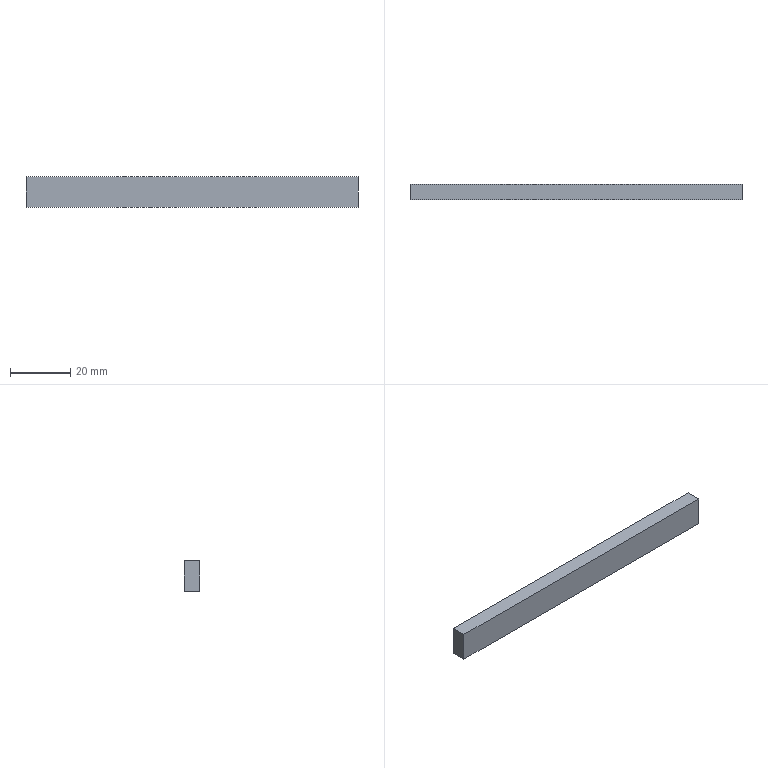Part | SolidWorks | features Extrusion 1, ICE 1 | 1 solid | 12 faces | box 110 x 5 x 10 mm | volume 5325 mm3 | plane 8 | cylinder 4 | commonest cylinder face diameters 6 x4
STEP:
#1=CARTESIAN_POINT('',(-49.,1.9,-3.));
#2=VERTEX_POINT('',#1);
#3=CARTESIAN_POINT('',(-49.,1.9,3.));
#4=VERTEX_POINT('',#3);
#5=CARTESIAN_POINT('',(-49.,1.9,0.));
#6=DIRECTION('',(0.,1.,0.));
#7=DIRECTION('',(0.,0.,1.));
#8=AXIS2_PLACEMENT_3D('',#5,#6,#7);
#9=CIRCLE('',#8,3.);
#10=EDGE_CURVE('',#2,#4,#9,.T.);
#11=ORIENTED_EDGE('',*,*,#10,.F.);
#12=CARTESIAN_POINT('',(-49.,5.,-3.));
#13=VERTEX_POINT('',#12);
#14=CARTESIAN_POINT('',(-49.,1.9,-3.));
#15=DIRECTION('',(0.,1.,0.));
#16=VECTOR('',#15,1000.);
#17=LINE('',#14,#16);
#18=EDGE_CURVE('',#2,#13,#17,.T.);
#19=ORIENTED_EDGE('',*,*,#18,.T.);
#20=CARTESIAN_POINT('',(-49.,5.,3.));
#21=VERTEX_POINT('',#20);
#22=CARTESIAN_POINT('',(-49.,5.,0.));
#23=DIRECTION('',(0.,1.,0.));
#24=DIRECTION('',(0.,0.,1.));
#25=AXIS2_PLACEMENT_3D('',#22,#23,#24);
#26=CIRCLE('',#25,3.);
#27=EDGE_CURVE('',#13,#21,#26,.T.);
#28=ORIENTED_EDGE('',*,*,#27,.T.);
#29=CARTESIAN_POINT('',(-49.,1.9,3.));
#30=DIRECTION('',(0.,1.,0.));
#31=VECTOR('',#30,1000.);
#32=LINE('',#29,#31);
#33=EDGE_CURVE('',#4,#21,#32,.T.);
#34=ORIENTED_EDGE('',*,*,#33,.F.);
#35=EDGE_LOOP('',(#11,#19,#28,#34));
#36=FACE_OUTER_BOUND('',#35,.T.);
#37=CARTESIAN_POINT('',(-49.,1.9,0.));
#38=DIRECTION('',(0.,1.,0.));
#39=DIRECTION('',(0.,0.,1.));
#40=AXIS2_PLACEMENT_3D('',#37,#38,#39);
#41=CYLINDRICAL_SURFACE('',#40,3.);
#42=ADVANCED_FACE('',(#36),#41,.F.);
#43=CARTESIAN_POINT('',(49.,1.9,-3.));
#44=VERTEX_POINT('',#43);
#45=CARTESIAN_POINT('',(49.,1.9,3.));
#46=VERTEX_POINT('',#45);
#47=CARTESIAN_POINT('',(49.,1.9,0.));
#48=DIRECTION('',(0.,1.,0.));
#49=DIRECTION('',(0.,0.,1.));
#50=AXIS2_PLACEMENT_3D('',#47,#48,#49);
#51=CIRCLE('',#50,3.);
#52=EDGE_CURVE('',#44,#46,#51,.T.);
#53=ORIENTED_EDGE('',*,*,#52,.F.);
#54=CARTESIAN_POINT('',(49.,5.,-3.));
#55=VERTEX_POINT('',#54);
#56=CARTESIAN_POINT('',(49.,1.9,-3.));
#57=DIRECTION('',(0.,1.,0.));
#58=VECTOR('',#57,1000.);
#59=LINE('',#56,#58);
#60=EDGE_CURVE('',#44,#55,#59,.T.);
#61=ORIENTED_EDGE('',*,*,#60,.T.);
#62=CARTESIAN_POINT('',(49.,5.,3.));
#63=VERTEX_POINT('',#62);
#64=CARTESIAN_POINT('',(49.,5.,0.));
#65=DIRECTION('',(0.,1.,0.));
#66=DIRECTION('',(0.,0.,1.));
#67=AXIS2_PLACEMENT_3D('',#64,#65,#66);
#68=CIRCLE('',#67,3.);
#69=EDGE_CURVE('',#55,#63,#68,.T.);
#70=ORIENTED_EDGE('',*,*,#69,.T.);
#71=CARTESIAN_POINT('',(49.,1.9,3.));
#72=DIRECTION('',(0.,1.,0.));
#73=VECTOR('',#72,1000.);
#74=LINE('',#71,#73);
#75=EDGE_CURVE('',#46,#63,#74,.T.);
#76=ORIENTED_EDGE('',*,*,#75,.F.);
#77=EDGE_LOOP('',(#53,#61,#70,#76));
#78=FACE_OUTER_BOUND('',#77,.T.);
#79=CARTESIAN_POINT('',(49.,1.9,0.));
#80=DIRECTION('',(0.,1.,0.));
#81=DIRECTION('',(0.,0.,1.));
#82=AXIS2_PLACEMENT_3D('',#79,#80,#81);
#83=CYLINDRICAL_SURFACE('',#82,3.);
#84=ADVANCED_FACE('',(#78),#83,.F.);
#85=CARTESIAN_POINT('',(55.,0.,5.));
#86=VERTEX_POINT('',#85);
#87=CARTESIAN_POINT('',(55.,0.,-5.));
#88=VERTEX_POINT('',#87);
#89=CARTESIAN_POINT('',(55.,0.,-5.));
#90=DIRECTION('',(0.,0.,-1.));
#91=VECTOR('',#90,1000.);
#92=LINE('',#89,#91);
#93=EDGE_CURVE('',#86,#88,#92,.T.);
#94=ORIENTED_EDGE('',*,*,#93,.T.);
#95=CARTESIAN_POINT('',(55.,5.,-5.));
#96=VERTEX_POINT('',#95);
#97=CARTESIAN_POINT('',(55.,5.,-5.));
#98=DIRECTION('',(0.,-1.,0.));
#99=VECTOR('',#98,1000.);
#100=LINE('',#97,#99);
#101=EDGE_CURVE('',#96,#88,#100,.T.);
#102=ORIENTED_EDGE('',*,*,#101,.F.);
#103=CARTESIAN_POINT('',(55.,5.,5.));
#104=VERTEX_POINT('',#103);
#105=CARTESIAN_POINT('',(55.,5.,-5.));
#106=DIRECTION('',(0.,0.,-1.));
#107=VECTOR('',#106,1000.);
#108=LINE('',#105,#107);
#109=EDGE_CURVE('',#104,#96,#108,.T.);
#110=ORIENTED_EDGE('',*,*,#109,.F.);
#111=CARTESIAN_POINT('',(55.,5.,5.));
#112=DIRECTION('',(0.,-1.,0.));
#113=VECTOR('',#112,1000.);
#114=LINE('',#111,#113);
#115=EDGE_CURVE('',#104,#86,#114,.T.);
#116=ORIENTED_EDGE('',*,*,#115,.T.);
#117=EDGE_LOOP('',(#94,#102,#110,#116));
#118=FACE_OUTER_BOUND('',#117,.T.);
#119=CARTESIAN_POINT('',(55.,5.,-5.));
#120=DIRECTION('',(-1.,0.,0.));
#121=DIRECTION('',(0.,0.,1.));
#122=AXIS2_PLACEMENT_3D('',#119,#120,#121);
#123=PLANE('',#122);
#124=ADVANCED_FACE('',(#118),#123,.F.);
#125=CARTESIAN_POINT('',(-55.,0.,-5.));
#126=VERTEX_POINT('',#125);
#127=CARTESIAN_POINT('',(-55.,0.,-5.));
#128=DIRECTION('',(-1.,0.,0.));
#129=VECTOR('',#128,1000.);
#130=LINE('',#127,#129);
#131=EDGE_CURVE('',#88,#126,#130,.T.);
#132=ORIENTED_EDGE('',*,*,#131,.T.);
#133=CARTESIAN_POINT('',(-55.,5.,-5.));
#134=VERTEX_POINT('',#133);
#135=CARTESIAN_POINT('',(-55.,5.,-5.));
#136=DIRECTION('',(0.,-1.,0.));
#137=VECTOR('',#136,1000.);
#138=LINE('',#135,#137);
#139=EDGE_CURVE('',#134,#126,#138,.T.);
#140=ORIENTED_EDGE('',*,*,#139,.F.);
#141=CARTESIAN_POINT('',(-55.,5.,-5.));
#142=DIRECTION('',(-1.,0.,0.));
#143=VECTOR('',#142,1000.);
#144=LINE('',#141,#143);
#145=EDGE_CURVE('',#96,#134,#144,.T.);
#146=ORIENTED_EDGE('',*,*,#145,.F.);
#147=ORIENTED_EDGE('',*,*,#101,.T.);
#148=EDGE_LOOP('',(#132,#140,#146,#147));
#149=FACE_OUTER_BOUND('',#148,.T.);
#150=CARTESIAN_POINT('',(-55.,5.,-5.));
#151=DIRECTION('',(0.,0.,1.));
#152=DIRECTION('',(1.,0.,0.));
#153=AXIS2_PLACEMENT_3D('',#150,#151,#152);
#154=PLANE('',#153);
#155=ADVANCED_FACE('',(#149),#154,.F.);
#156=CARTESIAN_POINT('',(-55.,0.,5.));
#157=VERTEX_POINT('',#156);
#158=CARTESIAN_POINT('',(-55.,0.,-5.));
#159=DIRECTION('',(0.,0.,1.));
#160=VECTOR('',#159,1000.);
#161=LINE('',#158,#160);
#162=EDGE_CURVE('',#126,#157,#161,.T.);
#163=ORIENTED_EDGE('',*,*,#162,.T.);
#164=CARTESIAN_POINT('',(-55.,5.,5.));
#165=VERTEX_POINT('',#164);
#166=CARTESIAN_POINT('',(-55.,5.,5.));
#167=DIRECTION('',(0.,-1.,0.));
#168=VECTOR('',#167,1000.);
#169=LINE('',#166,#168);
#170=EDGE_CURVE('',#165,#157,#169,.T.);
#171=ORIENTED_EDGE('',*,*,#170,.F.);
#172=CARTESIAN_POINT('',(-55.,5.,-5.));
#173=DIRECTION('',(0.,0.,1.));
#174=VECTOR('',#173,1000.);
#175=LINE('',#172,#174);
#176=EDGE_CURVE('',#134,#165,#175,.T.);
#177=ORIENTED_EDGE('',*,*,#176,.F.);
#178=ORIENTED_EDGE('',*,*,#139,.T.);
#179=EDGE_LOOP('',(#163,#171,#177,#178));
#180=FACE_OUTER_BOUND('',#179,.T.);
#181=CARTESIAN_POINT('',(-55.,5.,-5.));
#182=DIRECTION('',(1.,0.,0.));
#183=DIRECTION('',(0.,0.,-1.));
#184=AXIS2_PLACEMENT_3D('',#181,#182,#183);
#185=PLANE('',#184);
#186=ADVANCED_FACE('',(#180),#185,.F.);
#187=CARTESIAN_POINT('',(-55.,0.,5.));
#188=DIRECTION('',(1.,0.,0.));
#189=VECTOR('',#188,1000.);
#190=LINE('',#187,#189);
#191=EDGE_CURVE('',#157,#86,#190,.T.);
#192=ORIENTED_EDGE('',*,*,#191,.T.);
#193=ORIENTED_EDGE('',*,*,#115,.F.);
#194=CARTESIAN_POINT('',(-55.,5.,5.));
#195=DIRECTION('',(1.,0.,0.));
#196=VECTOR('',#195,1000.);
#197=LINE('',#194,#196);
#198=EDGE_CURVE('',#165,#104,#197,.T.);
#199=ORIENTED_EDGE('',*,*,#198,.F.);
#200=ORIENTED_EDGE('',*,*,#170,.T.);
#201=EDGE_LOOP('',(#192,#193,#199,#200));
#202=FACE_OUTER_BOUND('',#201,.T.);
#203=CARTESIAN_POINT('',(-55.,5.,5.));
#204=DIRECTION('',(0.,0.,-1.));
#205=DIRECTION('',(-1.,0.,0.));
#206=AXIS2_PLACEMENT_3D('',#203,#204,#205);
#207=PLANE('',#206);
#208=ADVANCED_FACE('',(#202),#207,.F.);
#209=CARTESIAN_POINT('',(-49.,5.,0.));
#210=DIRECTION('',(0.,1.,0.));
#211=DIRECTION('',(0.,0.,1.));
#212=AXIS2_PLACEMENT_3D('',#209,#210,#211);
#213=CIRCLE('',#212,3.);
#214=EDGE_CURVE('',#21,#13,#213,.T.);
#215=ORIENTED_EDGE('',*,*,#214,.F.);
#216=ORIENTED_EDGE('',*,*,#27,.F.);
#217=EDGE_LOOP('',(#215,#216));
#218=FACE_BOUND('',#217,.T.);
#219=CARTESIAN_POINT('',(49.,5.,0.));
#220=DIRECTION('',(0.,1.,0.));
#221=DIRECTION('',(0.,0.,1.));
#222=AXIS2_PLACEMENT_3D('',#219,#220,#221);
#223=CIRCLE('',#222,3.);
#224=EDGE_CURVE('',#63,#55,#223,.T.);
#225=ORIENTED_EDGE('',*,*,#224,.F.);
#226=ORIENTED_EDGE('',*,*,#69,.F.);
#227=EDGE_LOOP('',(#225,#226));
#228=FACE_BOUND('',#227,.T.);
#229=ORIENTED_EDGE('',*,*,#109,.T.);
#230=ORIENTED_EDGE('',*,*,#145,.T.);
#231=ORIENTED_EDGE('',*,*,#176,.T.);
#232=ORIENTED_EDGE('',*,*,#198,.T.);
#233=EDGE_LOOP('',(#229,#230,#231,#232));
#234=FACE_OUTER_BOUND('',#233,.T.);
#235=CARTESIAN_POINT('',(0.,5.,0.));
#236=DIRECTION('',(0.,1.,0.));
#237=DIRECTION('',(0.,0.,1.));
#238=AXIS2_PLACEMENT_3D('',#235,#236,#237);
#239=PLANE('',#238);
#240=ADVANCED_FACE('',(#218,#228,#234),#239,.T.);
#241=ORIENTED_EDGE('',*,*,#93,.F.);
#242=ORIENTED_EDGE('',*,*,#191,.F.);
#243=ORIENTED_EDGE('',*,*,#162,.F.);
#244=ORIENTED_EDGE('',*,*,#131,.F.);
#245=EDGE_LOOP('',(#241,#242,#243,#244));
#246=FACE_OUTER_BOUND('',#245,.T.);
#247=CARTESIAN_POINT('',(0.,0.,0.));
#248=DIRECTION('',(0.,1.,0.));
#249=DIRECTION('',(0.,0.,1.));
#250=AXIS2_PLACEMENT_3D('',#247,#248,#249);
#251=PLANE('',#250);
#252=ADVANCED_FACE('',(#246),#251,.F.);
#253=ORIENTED_EDGE('',*,*,#60,.F.);
#254=CARTESIAN_POINT('',(49.,1.9,0.));
#255=DIRECTION('',(0.,1.,0.));
#256=DIRECTION('',(0.,0.,1.));
#257=AXIS2_PLACEMENT_3D('',#254,#255,#256);
#258=CIRCLE('',#257,3.);
#259=EDGE_CURVE('',#46,#44,#258,.T.);
#260=ORIENTED_EDGE('',*,*,#259,.F.);
#261=ORIENTED_EDGE('',*,*,#75,.T.);
#262=ORIENTED_EDGE('',*,*,#224,.T.);
#263=EDGE_LOOP('',(#253,#260,#261,#262));
#264=FACE_OUTER_BOUND('',#263,.T.);
#265=CARTESIAN_POINT('',(49.,1.9,0.));
#266=DIRECTION('',(0.,1.,0.));
#267=DIRECTION('',(0.,0.,1.));
#268=AXIS2_PLACEMENT_3D('',#265,#266,#267);
#269=CYLINDRICAL_SURFACE('',#268,3.);
#270=ADVANCED_FACE('',(#264),#269,.F.);
#271=ORIENTED_EDGE('',*,*,#259,.T.);
#272=ORIENTED_EDGE('',*,*,#52,.T.);
#273=EDGE_LOOP('',(#271,#272));
#274=FACE_OUTER_BOUND('',#273,.T.);
#275=CARTESIAN_POINT('',(49.,1.9,0.));
#276=DIRECTION('',(0.,1.,0.));
#277=DIRECTION('',(0.,0.,1.));
#278=AXIS2_PLACEMENT_3D('',#275,#276,#277);
#279=PLANE('',#278);
#280=ADVANCED_FACE('',(#274),#279,.T.);
#281=ORIENTED_EDGE('',*,*,#18,.F.);
#282=CARTESIAN_POINT('',(-49.,1.9,0.));
#283=DIRECTION('',(0.,1.,0.));
#284=DIRECTION('',(0.,0.,1.));
#285=AXIS2_PLACEMENT_3D('',#282,#283,#284);
#286=CIRCLE('',#285,3.);
#287=EDGE_CURVE('',#4,#2,#286,.T.);
#288=ORIENTED_EDGE('',*,*,#287,.F.);
#289=ORIENTED_EDGE('',*,*,#33,.T.);
#290=ORIENTED_EDGE('',*,*,#214,.T.);
#291=EDGE_LOOP('',(#281,#288,#289,#290));
#292=FACE_OUTER_BOUND('',#291,.T.);
#293=CARTESIAN_POINT('',(-49.,1.9,0.));
#294=DIRECTION('',(0.,1.,0.));
#295=DIRECTION('',(0.,0.,1.));
#296=AXIS2_PLACEMENT_3D('',#293,#294,#295);
#297=CYLINDRICAL_SURFACE('',#296,3.);
#298=ADVANCED_FACE('',(#292),#297,.F.);
#299=ORIENTED_EDGE('',*,*,#287,.T.);
#300=ORIENTED_EDGE('',*,*,#10,.T.);
#301=EDGE_LOOP('',(#299,#300));
#302=FACE_OUTER_BOUND('',#301,.T.);
#303=CARTESIAN_POINT('',(-49.,1.9,0.));
#304=DIRECTION('',(0.,1.,0.));
#305=DIRECTION('',(0.,0.,1.));
#306=AXIS2_PLACEMENT_3D('',#303,#304,#305);
#307=PLANE('',#306);
#308=ADVANCED_FACE('',(#302),#307,.T.);
#309=CLOSED_SHELL('',(#42,#84,#124,#155,#186,#208,#240,#252,#270,#280,#298,#308));
#310=MANIFOLD_SOLID_BREP('',#309);
#311=CARTESIAN_POINT('',(0.,0.,0.));
#312=DIRECTION('',(0.,0.,1.));
#313=DIRECTION('',(1.,0.,0.));
#314=AXIS2_PLACEMENT_3D('',#311,#312,#313);
#315=(LENGTH_UNIT()NAMED_UNIT(*)SI_UNIT(.MILLI.,.METRE.));
#316=UNCERTAINTY_MEASURE_WITH_UNIT(LENGTH_MEASURE(0.00001),#315,'','');
#317=(NAMED_UNIT(*)PLANE_ANGLE_UNIT()SI_UNIT($,.RADIAN.));
#318=(NAMED_UNIT(*)SI_UNIT($,.STERADIAN.)SOLID_ANGLE_UNIT());
#319=(GEOMETRIC_REPRESENTATION_CONTEXT(3)GLOBAL_UNCERTAINTY_ASSIGNED_CONTEXT((#316))GLOBAL_UNIT_ASSIGNED_CONTEXT((#315,#317,#318))REPRESENTATION_CONTEXT('',''));
#320=ADVANCED_BREP_SHAPE_REPRESENTATION('',(#310,#314),#319);